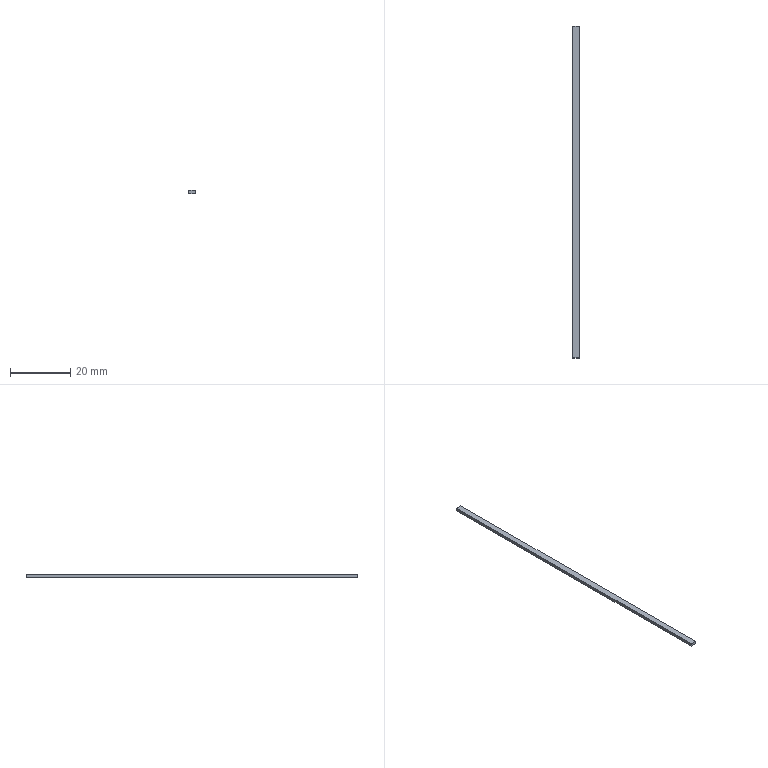Part | STEP file | lll_id930_x_t | 1 solid | 6 faces | box 2 x 110.066 x 1 mm | volume 220.133 mm3 | plane 6
STEP:
#1=CARTESIAN_POINT('',(366.009,-501.065,1.259));
#2=VERTEX_POINT('',#1);
#3=CARTESIAN_POINT('',(368.009,-501.065,1.259));
#4=VERTEX_POINT('',#3);
#5=CARTESIAN_POINT('',(367.009,-501.065,1.259));
#6=DIRECTION('',(1.,0.,0.));
#7=VECTOR('',#6,1.);
#8=LINE('',#5,#7);
#9=EDGE_CURVE('',#2,#4,#8,.T.);
#10=ORIENTED_EDGE('',*,*,#9,.F.);
#11=CARTESIAN_POINT('',(366.009,-390.999,1.259));
#12=VERTEX_POINT('',#11);
#13=CARTESIAN_POINT('',(366.009,-501.065,1.259));
#14=DIRECTION('',(0.,1.,0.));
#15=VECTOR('',#14,1.);
#16=LINE('',#13,#15);
#17=EDGE_CURVE('',#2,#12,#16,.T.);
#18=ORIENTED_EDGE('',*,*,#17,.T.);
#19=CARTESIAN_POINT('',(368.009,-390.999,1.259));
#20=VERTEX_POINT('',#19);
#21=CARTESIAN_POINT('',(367.009,-390.999,1.259));
#22=DIRECTION('',(1.,0.,0.));
#23=VECTOR('',#22,1.);
#24=LINE('',#21,#23);
#25=EDGE_CURVE('',#12,#20,#24,.T.);
#26=ORIENTED_EDGE('',*,*,#25,.T.);
#27=CARTESIAN_POINT('',(368.009,-501.065,1.259));
#28=DIRECTION('',(0.,1.,0.));
#29=VECTOR('',#28,1.);
#30=LINE('',#27,#29);
#31=EDGE_CURVE('',#4,#20,#30,.T.);
#32=ORIENTED_EDGE('',*,*,#31,.F.);
#33=EDGE_LOOP('',(#10,#18,#26,#32));
#34=FACE_OUTER_BOUND('',#33,.T.);
#35=CARTESIAN_POINT('',(367.009,-501.065,1.259));
#36=DIRECTION('',(0.,0.,-1.));
#37=DIRECTION('',(0.,1.,0.));
#38=AXIS2_PLACEMENT_3D('',#35,#36,#37);
#39=PLANE('',#38);
#40=ADVANCED_FACE('',(#34),#39,.T.);
#41=ORIENTED_EDGE('',*,*,#25,.F.);
#42=CARTESIAN_POINT('',(366.009,-390.999,2.259));
#43=VERTEX_POINT('',#42);
#44=CARTESIAN_POINT('',(366.009,-390.999,1.259));
#45=DIRECTION('',(0.,0.,1.));
#46=VECTOR('',#45,1.);
#47=LINE('',#44,#46);
#48=EDGE_CURVE('',#12,#43,#47,.T.);
#49=ORIENTED_EDGE('',*,*,#48,.T.);
#50=CARTESIAN_POINT('',(368.009,-390.999,2.259));
#51=VERTEX_POINT('',#50);
#52=CARTESIAN_POINT('',(367.009,-390.999,2.259));
#53=DIRECTION('',(1.,0.,0.));
#54=VECTOR('',#53,1.);
#55=LINE('',#52,#54);
#56=EDGE_CURVE('',#43,#51,#55,.T.);
#57=ORIENTED_EDGE('',*,*,#56,.T.);
#58=CARTESIAN_POINT('',(368.009,-390.999,1.259));
#59=DIRECTION('',(0.,0.,1.));
#60=VECTOR('',#59,1.);
#61=LINE('',#58,#60);
#62=EDGE_CURVE('',#20,#51,#61,.T.);
#63=ORIENTED_EDGE('',*,*,#62,.F.);
#64=EDGE_LOOP('',(#41,#49,#57,#63));
#65=FACE_OUTER_BOUND('',#64,.T.);
#66=CARTESIAN_POINT('',(367.009,-390.999,1.259));
#67=DIRECTION('',(0.,1.,0.));
#68=DIRECTION('',(0.,0.,1.));
#69=AXIS2_PLACEMENT_3D('',#66,#67,#68);
#70=PLANE('',#69);
#71=ADVANCED_FACE('',(#65),#70,.T.);
#72=ORIENTED_EDGE('',*,*,#56,.F.);
#73=CARTESIAN_POINT('',(366.009,-501.065,2.259));
#74=VERTEX_POINT('',#73);
#75=CARTESIAN_POINT('',(366.009,-501.065,2.259));
#76=DIRECTION('',(0.,1.,0.));
#77=VECTOR('',#76,1.);
#78=LINE('',#75,#77);
#79=EDGE_CURVE('',#74,#43,#78,.T.);
#80=ORIENTED_EDGE('',*,*,#79,.F.);
#81=CARTESIAN_POINT('',(368.009,-501.065,2.259));
#82=VERTEX_POINT('',#81);
#83=CARTESIAN_POINT('',(367.009,-501.065,2.259));
#84=DIRECTION('',(1.,0.,0.));
#85=VECTOR('',#84,1.);
#86=LINE('',#83,#85);
#87=EDGE_CURVE('',#74,#82,#86,.T.);
#88=ORIENTED_EDGE('',*,*,#87,.T.);
#89=CARTESIAN_POINT('',(368.009,-501.065,2.259));
#90=DIRECTION('',(0.,1.,0.));
#91=VECTOR('',#90,1.);
#92=LINE('',#89,#91);
#93=EDGE_CURVE('',#82,#51,#92,.T.);
#94=ORIENTED_EDGE('',*,*,#93,.T.);
#95=EDGE_LOOP('',(#72,#80,#88,#94));
#96=FACE_OUTER_BOUND('',#95,.T.);
#97=CARTESIAN_POINT('',(367.009,-501.065,2.259));
#98=DIRECTION('',(0.,0.,-1.));
#99=DIRECTION('',(0.,1.,0.));
#100=AXIS2_PLACEMENT_3D('',#97,#98,#99);
#101=PLANE('',#100);
#102=ADVANCED_FACE('',(#96),#101,.F.);
#103=CARTESIAN_POINT('',(366.009,-501.065,1.259));
#104=DIRECTION('',(0.,0.,1.));
#105=VECTOR('',#104,1.);
#106=LINE('',#103,#105);
#107=EDGE_CURVE('',#2,#74,#106,.T.);
#108=ORIENTED_EDGE('',*,*,#107,.F.);
#109=ORIENTED_EDGE('',*,*,#9,.T.);
#110=CARTESIAN_POINT('',(368.009,-501.065,1.259));
#111=DIRECTION('',(0.,0.,1.));
#112=VECTOR('',#111,1.);
#113=LINE('',#110,#112);
#114=EDGE_CURVE('',#4,#82,#113,.T.);
#115=ORIENTED_EDGE('',*,*,#114,.T.);
#116=ORIENTED_EDGE('',*,*,#87,.F.);
#117=EDGE_LOOP('',(#108,#109,#115,#116));
#118=FACE_OUTER_BOUND('',#117,.T.);
#119=CARTESIAN_POINT('',(367.009,-501.065,1.259));
#120=DIRECTION('',(0.,1.,0.));
#121=DIRECTION('',(0.,0.,1.));
#122=AXIS2_PLACEMENT_3D('',#119,#120,#121);
#123=PLANE('',#122);
#124=ADVANCED_FACE('',(#118),#123,.F.);
#125=ORIENTED_EDGE('',*,*,#93,.F.);
#126=ORIENTED_EDGE('',*,*,#114,.F.);
#127=ORIENTED_EDGE('',*,*,#31,.T.);
#128=ORIENTED_EDGE('',*,*,#62,.T.);
#129=EDGE_LOOP('',(#125,#126,#127,#128));
#130=FACE_OUTER_BOUND('',#129,.T.);
#131=CARTESIAN_POINT('',(368.009,-501.065,1.259));
#132=DIRECTION('',(1.,0.,0.));
#133=DIRECTION('',(0.,0.,-1.));
#134=AXIS2_PLACEMENT_3D('',#131,#132,#133);
#135=PLANE('',#134);
#136=ADVANCED_FACE('',(#130),#135,.T.);
#137=ORIENTED_EDGE('',*,*,#79,.T.);
#138=ORIENTED_EDGE('',*,*,#48,.F.);
#139=ORIENTED_EDGE('',*,*,#17,.F.);
#140=ORIENTED_EDGE('',*,*,#107,.T.);
#141=EDGE_LOOP('',(#137,#138,#139,#140));
#142=FACE_OUTER_BOUND('',#141,.T.);
#143=CARTESIAN_POINT('',(366.009,-501.065,1.259));
#144=DIRECTION('',(1.,0.,0.));
#145=DIRECTION('',(0.,0.,-1.));
#146=AXIS2_PLACEMENT_3D('',#143,#144,#145);
#147=PLANE('',#146);
#148=ADVANCED_FACE('',(#142),#147,.F.);
#149=CLOSED_SHELL('',(#40,#71,#102,#124,#136,#148));
#150=MANIFOLD_SOLID_BREP('',#149);
#151=(LENGTH_UNIT()NAMED_UNIT(*)SI_UNIT(.MILLI.,.METRE.));
#152=UNCERTAINTY_MEASURE_WITH_UNIT(LENGTH_MEASURE(0.00002),#151,'','');
#153=(NAMED_UNIT(*)PLANE_ANGLE_UNIT()SI_UNIT($,.RADIAN.));
#154=PLANE_ANGLE_MEASURE_WITH_UNIT(PLANE_ANGLE_MEASURE(0.01745),#153);
#155=DIMENSIONAL_EXPONENTS(0.,0.,0.,0.,0.,0.,0.);
#156=(CONVERSION_BASED_UNIT('DEGREE',#154)NAMED_UNIT(#155)PLANE_ANGLE_UNIT());
#157=(NAMED_UNIT(*)SI_UNIT($,.STERADIAN.)SOLID_ANGLE_UNIT());
#158=(GEOMETRIC_REPRESENTATION_CONTEXT(3)GLOBAL_UNCERTAINTY_ASSIGNED_CONTEXT((#152))GLOBAL_UNIT_ASSIGNED_CONTEXT((#151,#156,#157))REPRESENTATION_CONTEXT('',''));
#159=ADVANCED_BREP_SHAPE_REPRESENTATION('',(#150),#158);